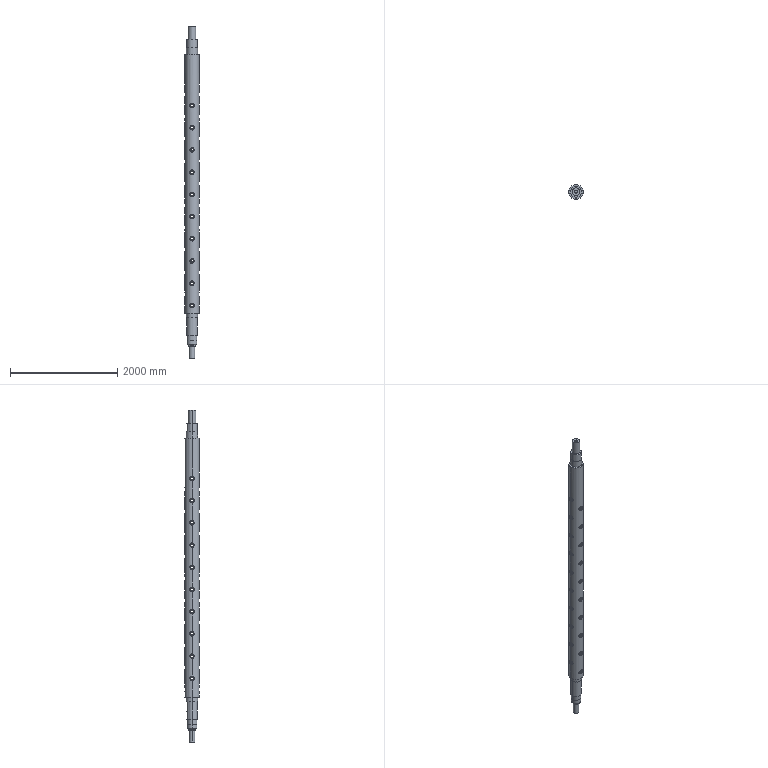Part | SolidWorks | features ICE 16, HoleWzd 4, LPattern 4, MirrorPattern 4, Chamfer 2, CombineBodies 2, Fillet 2, MoveFace 2, RefAxis 2, CirPattern 1, DeleteBody 1, Extrusion 1, MoveCopyBody 1, Revolution 1, Split 1, WeldmentFeature 1 | 5 solids | 273 faces | box 265 x 265 x 6190 mm | volume 134783572 mm3 | cylinder 198 | plane 59 | cone 12 | torus 4 | commonest cylinder face diameters 50 x82 85 x80 207 x8 8.5 x6 180 x4 200 x4